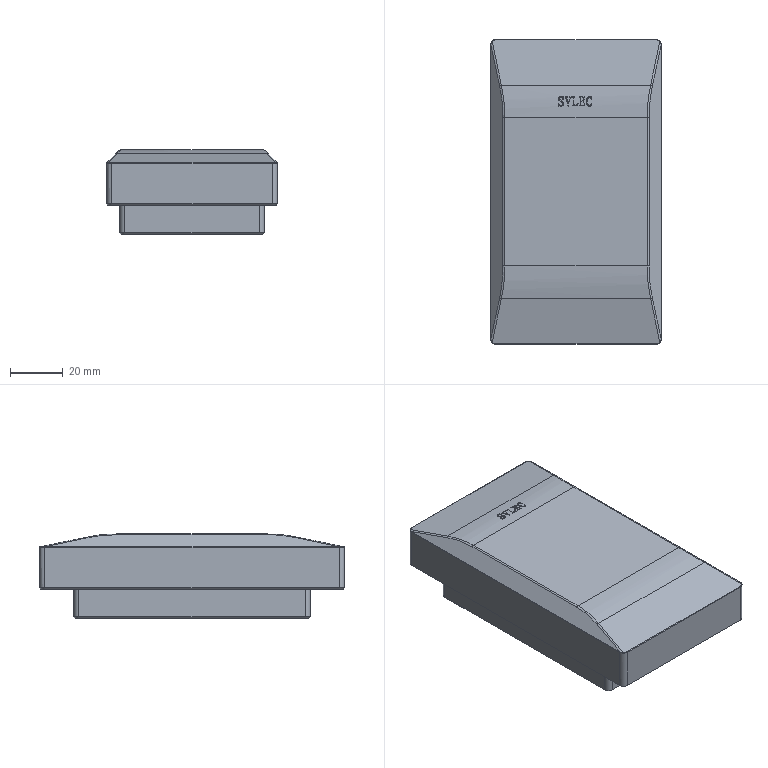Part | SolidWorks | features Fillet 5, Chamfer 3, ICE 2, Emboss 1, Extrusion 1 | 1 solid | 368 faces | box 65 x 116 x 32 mm | volume 202668 mm3 | plane 194 | spline 141 | cylinder 25 | cone 8 | commonest cylinder face diameters 4 x8 2 x6 119.8 x5 0.4 x4 120 x2